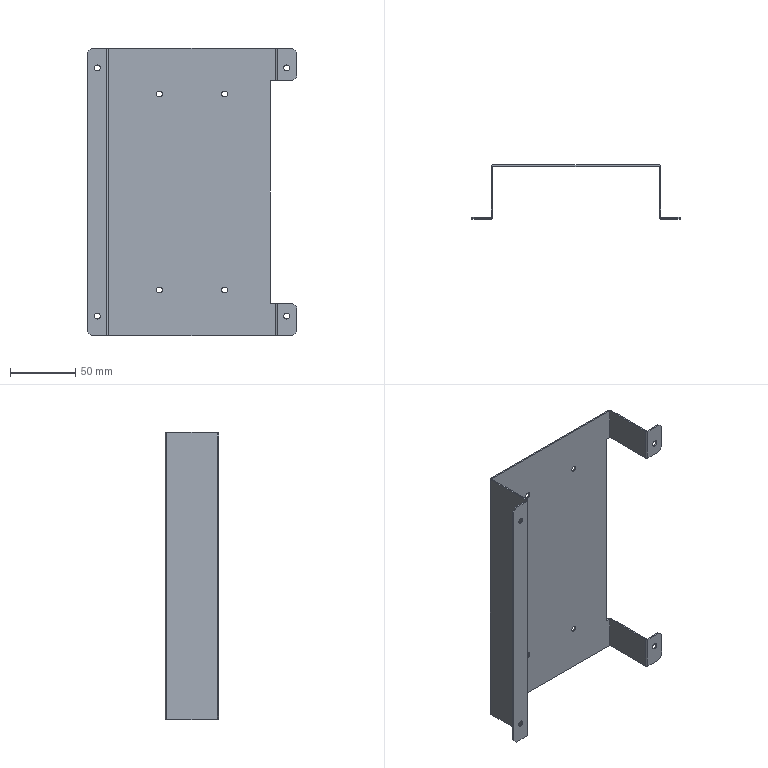Part | SolidWorks | features ICE 3, CornerTrim 1, FlatPattern 1, SMBaseFlange 1, SheetMetal 1 | 1 solid | 80 faces | box 160 x 41 x 220 mm | volume 42307 mm3 | plane 52 | cylinder 28 | commonest cylinder face diameters 4.5 x16 0.2 x6 2.2 x6